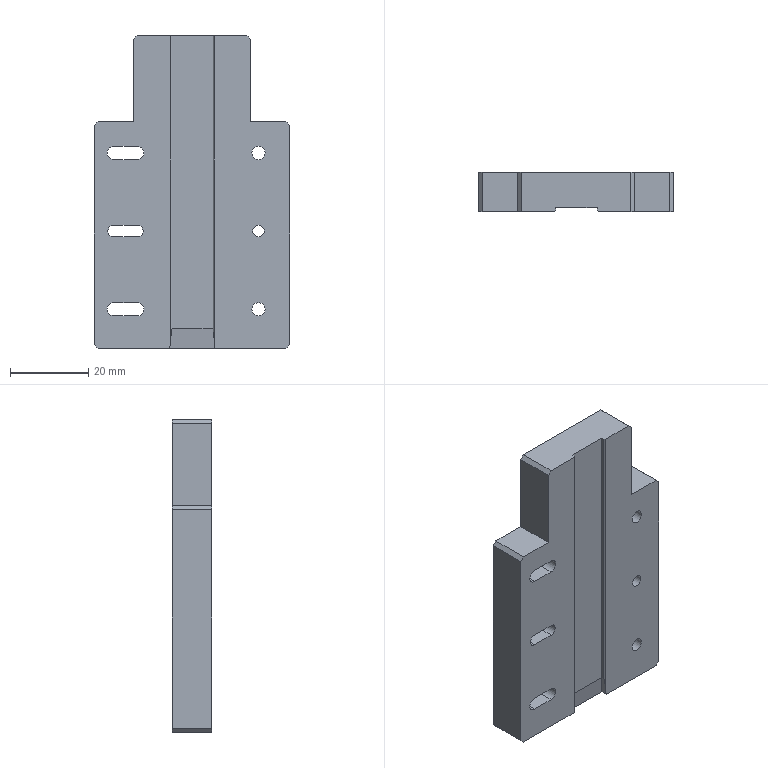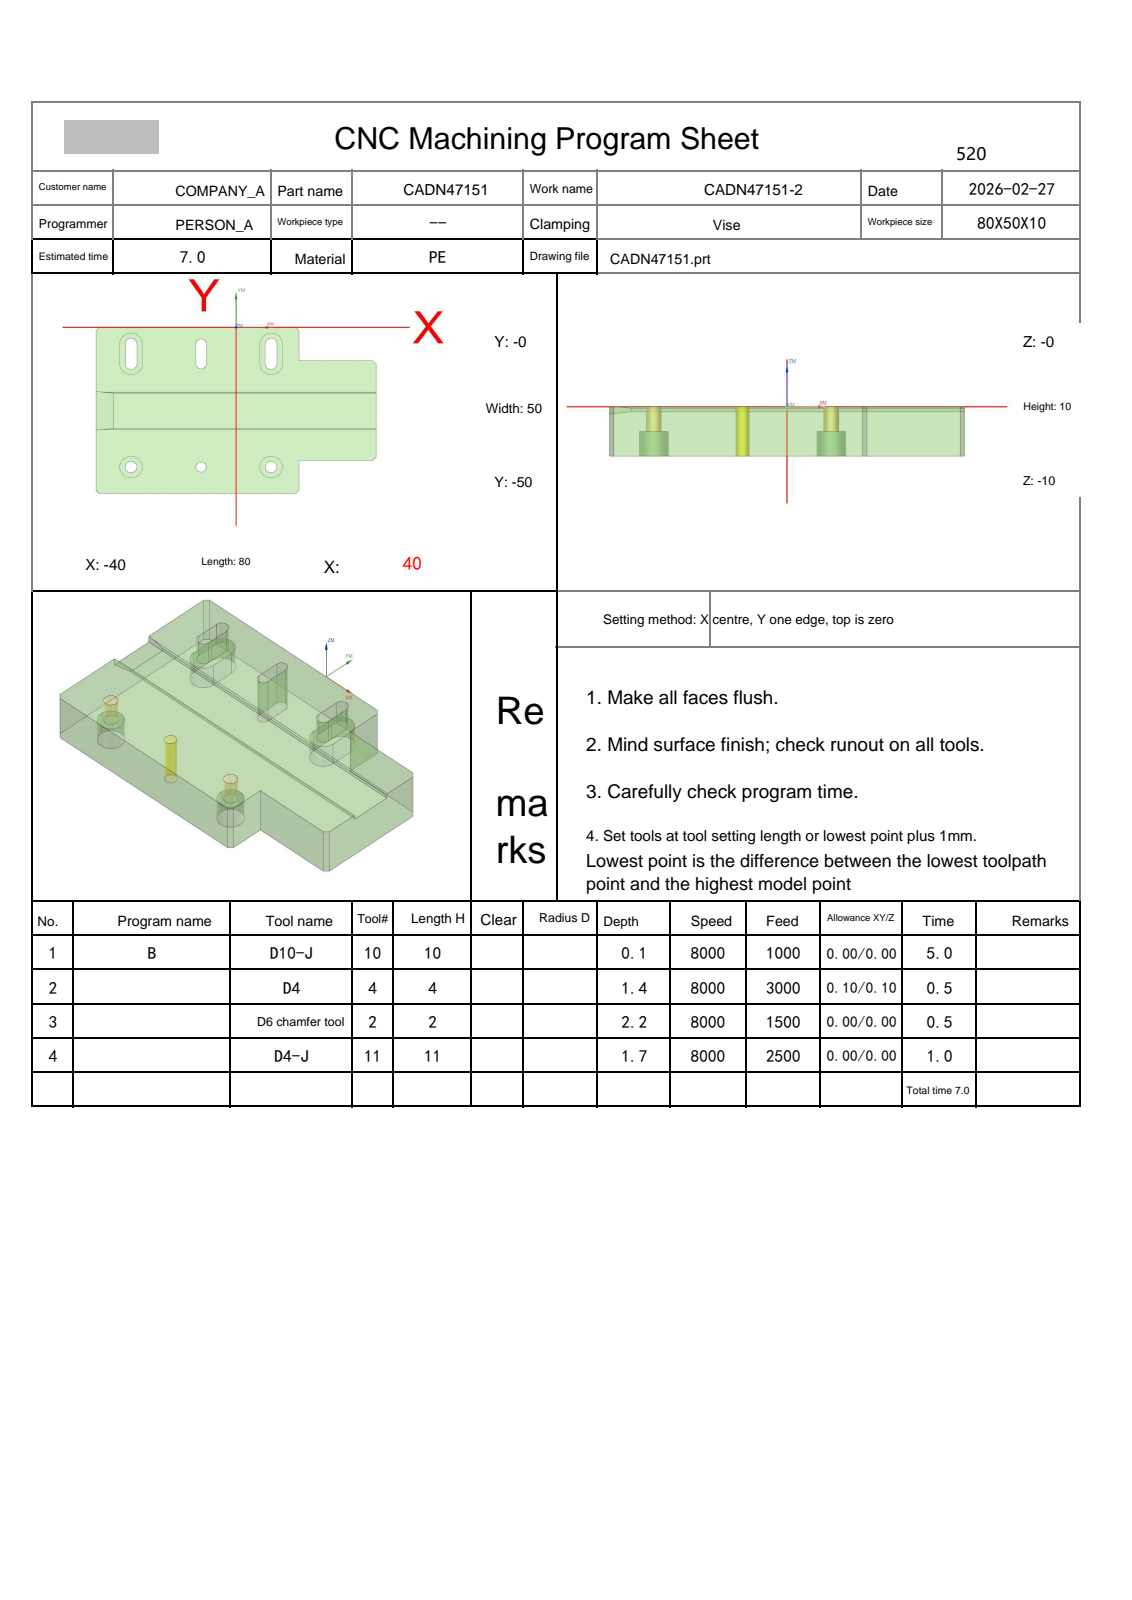NC program | NX | posted by the shop | part box 50 x 10 x 80 mm
Whole program:
%
O0001
(Machine time: 7.76 MIN)
(===Total Tool:4===)
(T10=D10-J  D=10.  R=0.   D-  H10 Z=-0.   )
(T4=D4      D=4.   R=0.   D-  H04 Z=-1.4  )
(T2=D6 chamfer tool   D=6.   R=0.   D-  H02 Z=-2.2  )
(T11=D4-J   D=4.   R=0.   D11 H11 Z=-1.72 )
G80 G90 G17 G49 G40
G91 G28 Z0
M01
N1 T10 M06
(D10-J  D=10. R=0. H=10 ce=0.00 di=0.10)
G00 G90 G54 X-57. Y-16.375 M03 S8000
G43 H10 Z50.
M08
Z3.525
G01 Z1.525 F1000.
X-45. Y-4.375
X-35.625 Y5.
X-26.25
X-45. Y-13.75
Y-23.125
X-16.875 Y5.
X-7.5
X-45. Y-32.5
Y-41.875
X1.875 Y5.
X11.25
X-45. Y-51.25
Y-55.
X-39.375
X20.625 Y5.
X30.
X-30. Y-55.
X-20.625
X39.375 Y5.
X45.
Y1.25
X-11.25 Y-55.
X-1.875
X45. Y-8.125
Y-17.5
X7.5 Y-55.
X16.875
X45. Y-26.875
Y-36.25
X26.25 Y-55.
X35.625
X45. Y-45.625
X57. Y-33.625
Z3.525
G00 Z5.
X-57. Y-16.375
Z3.05
G01 Z1.05
X-45. Y-4.375
X-35.625 Y5.
X-26.25
X-45. Y-13.75
Y-23.125
X-16.875 Y5.
X-7.5
X-45. Y-32.5
Y-41.875
X1.875 Y5.
X11.25
X-45. Y-51.25
Y-55.
X-39.375
X20.625 Y5.
X30.
X-30. Y-55.
X-20.625
X39.375 Y5.
X45.
Y1.25
X-11.25 Y-55.
X-1.875
X45. Y-8.125
Y-17.5
X7.5 Y-55.
X16.875
X45. Y-26.875
Y-36.25
X26.25 Y-55.
X35.625
X45. Y-45.625
X57. Y-33.625
Z3.05
G00 Z4.525
X-57. Y-16.375
Z2.575
G01 Z.575
X-45. Y-4.375
X-35.625 Y5.
X-26.25
X-45. Y-13.75
Y-23.125
X-16.875 Y5.
X-7.5
X-45. Y-32.5
Y-41.875
X1.875 Y5.
X11.25
X-45. Y-51.25
Y-55.
X-39.375
X20.625 Y5.
X30.
X-30. Y-55.
X-20.625
X39.375 Y5.
X45.
Y1.25
X-11.25 Y-55.
X-1.875
X45. Y-8.125
Y-17.5
X7.5 Y-55.
X16.875
X45. Y-26.875
Y-36.25
X26.25 Y-55.
X35.625
X45. Y-45.625
X57. Y-33.625
Z2.575
G00 Z4.05
X-57. Y-16.375
Z2.1
G01 Z.1
X-45. Y-4.375
X-35.625 Y5.
X-26.25
X-45. Y-13.75
Y-23.125
X-16.875 Y5.
X-7.5
X-45. Y-32.5
Y-41.875
X1.875 Y5.
X11.25
X-45. Y-51.25
Y-55.
X-39.375
X20.625 Y5.
X30.
X-30. Y-55.
X-20.625
X39.375 Y5.
X45.
Y1.25
X-11.25 Y-55.
X-1.875
X45. Y-8.125
Y-17.5
X7.5 Y-55.
X16.875
X45. Y-26.875
Y-36.25
X26.25 Y-55.
X35.625
X45. Y-45.625
X57. Y-33.625
Z2.1
G00 Z50.
G00 G90 X-57. Y-16.375 M03 S8000
Z50.
Z2.
G01 Z0.0 F1000.
X-45. Y-4.375
X-35.625 Y5.
X-26.25
X-45. Y-13.75
Y-23.125
X-16.875 Y5.
X-7.5
X-45. Y-32.5
Y-41.875
X1.875 Y5.
X11.25
X-45. Y-51.25
Y-55.
X-39.375
X20.625 Y5.
X30.
X-30. Y-55.
X-20.625
X39.375 Y5.
X45.
Y1.25
X-11.25 Y-55.
X-1.875
X45. Y-8.125
Y-17.5
X7.5 Y-55.
X16.875
X45. Y-26.875
Y-36.25
X26.25 Y-55.
X35.625
X45. Y-45.625
X57. Y-33.625
Z2.
G00 Z50.
G91 G28 Z0.0
M05
M09
G91 G28 Z0.0
M01
N2 T04 M06
(D4  D=4. R=0. H=04 ce=0.10 di=0.10)
G00 G90 G54 X-44.889 Y-27.898 M03 S8000
G43 H04 Z11.8
M08
Z1.
G01 Z-.2 F3000.
X-44.888
G03 X-42.088 Y-25.099 I0.0 J2.8
G01 X-42.086 Y-19.925
X-42.101 Y-19.852
X-42.027 Y-19.848
G03 X-40.209 Y-21.39 I2.027 J.548
G01 X-39.986 Y-21.412
X-39.995 Y-21.49
X-39.913 Y-21.499
X-38.72 Y-21.617
X-38.57 Y-21.632
X-38.138 Y-21.672
X-37.956 Y-21.651
X-37.598
X-35.691 Y-21.841
X39.92
X40.
X40.08
Y-22.017
Y-28.183
Y-28.359
X40.
X39.92
X-35.691
X-37.513 Y-28.541
X-37.998
X-38.186 Y-28.529
X-38.72 Y-28.583
X-39.914 Y-28.701
X-39.995 Y-28.71
X-39.986 Y-28.788
X-40.209 Y-28.81
G03 X-42.024 Y-30.341 I.209 J-2.09
G01 X-42.082 Y-30.339
X-42.059 Y-30.286
X-42.09 Y-30.058
X-42.089 Y-26.617
G02 X-41.884 Y-26.269 I.4 J0.0
G01 X-39.449 Y-24.906
G03 X-39.266 Y-24.687 I-.195 J.349
G02 X-38.888 Y-24.417 I.378 J-.13
G01 X-38.849 Y-24.419
X-38.465 Y-24.457
G03 X-38.259 Y-24.47 I.287 J2.866
G01 X-38.148 Y-24.472
G03 X-37.819 Y-24.453 I0.0 J2.88
G01 X-35.83 Y-24.641
X36.881
G02 X37.28 Y-25.041 I-.001 J-.4
G01 Y-25.159
G02 X36.881 Y-25.559 I-.4 J.001
G01 X-35.83
X-37.672 Y-25.741
X-37.875
G03 X-38.147 Y-25.728 I-.271 J-2.867
G01 X-38.22 Y-25.729
G03 X-38.465 Y-25.743 I.044 J-2.88
G01 X-38.849 Y-25.781
X-38.888 Y-25.783
G02 X-39.288 Y-25.384 I0.0 J.4
G01 Y-24.884
Y-24.883
G03 X-42.087 Y-22.083 I-2.8 J0.0
G01 X-44.887 Y-22.082
Z1.
G00 Z3.
G01 X-44.889 Y-27.898 F6000.
G00 Z.8
G01 Z-.4 F3000.
X-44.888
G03 X-42.088 Y-25.099 I0.0 J2.8
G01 X-42.086 Y-19.925
X-42.101 Y-19.852
X-42.027 Y-19.848
G03 X-40.209 Y-21.39 I2.027 J.548
G01 X-40.068 Y-21.404
X-40.077 Y-21.48
X-39.913 Y-21.499
X-38.72 Y-21.617
X-38.571 Y-21.632
X-38.137 Y-21.671
X-37.956 Y-21.651
X-37.598
X-35.209 Y-21.89
G03 X-35. Y-21.9 I.209 J2.09
G01 X39.92
X40.
X40.008
X40.08
Y-22.017
Y-28.183
Y-28.3
X40.004
X40.
X39.92
X-35.
G03 X-35.209 Y-28.31 I0.0 J-2.1
G01 X-37.513 Y-28.541
X-37.998
X-38.186 Y-28.529
X-38.72 Y-28.583
X-39.914 Y-28.701
X-40.077 Y-28.72
X-40.068 Y-28.796
X-40.209 Y-28.81
G03 X-42.024 Y-30.341 I.209 J-2.09
G01 X-42.082 Y-30.339
X-42.059 Y-30.286
X-42.09 Y-30.058
X-42.089 Y-26.617
G02 X-41.884 Y-26.269 I.4 J0.0
G01 X-39.449 Y-24.906
G03 X-39.266 Y-24.687 I-.196 J.349
G02 X-38.888 Y-24.417 I.378 J-.13
G01 X-38.849 Y-24.419
X-38.465 Y-24.457
G03 X-38.259 Y-24.47 I.287 J2.866
G01 X-38.118 Y-24.474
G03 X-37.756 Y-24.451 I0.0 J2.885
G01 X-35.488 Y-24.676
G03 X-35. Y-24.7 I.488 J4.876
G01 X36.881
G02 X37.28 Y-25.1 I-.001 J-.4
X36.881 Y-25.5 I-.4 J0.0
G01 X-35.
G03 X-35.488 Y-25.524 I0.0 J-4.9
G01 X-37.895 Y-25.739
G03 X-38.147 Y-25.728 I-.252 J-2.869
G01 X-38.22 Y-25.729
G03 X-38.465 Y-25.743 I.044 J-2.88
G01 X-38.849 Y-25.781
X-38.888 Y-25.783
G02 X-39.288 Y-25.384 I0.0 J.4
G01 Y-24.884
Y-24.883
G03 X-42.087 Y-22.083 I-2.8 J0.0
G01 X-44.887 Y-22.082
Z.8
G00 Z2.8
G01 X-44.889 Y-27.898 F6000.
G00 Z.6
G01 Z-.6 F3000.
X-44.888
G03 X-42.088 Y-25.099 I0.0 J2.8
G01 X-42.086 Y-19.925
X-42.101 Y-19.852
X-42.027 Y-19.848
G03 X-40.149 Y-21.396 I2.028 J.548
G01 X-40.158 Y-21.47
X-39.913 Y-21.499
X-38.72 Y-21.617
X-38.571 Y-21.632
X-38.138 Y-21.672
X-37.956 Y-21.651
X-37.598
X-35.209 Y-21.89
G03 X-35. Y-21.9 I.209 J2.09
G01 X39.92
X40.
X40.008
X40.08
Y-22.017
Y-28.183
Y-28.3
X40.004
X40.
X39.92
X-35.
G03 X-35.209 Y-28.31 I0.0 J-2.1
G01 X-37.513 Y-28.541
X-37.998
X-38.186 Y-28.529
X-38.72 Y-28.583
X-39.914 Y-28.701
X-40.158 Y-28.73
X-40.149 Y-28.804
X-40.209 Y-28.81
G03 X-42.024 Y-30.341 I.209 J-2.09
G01 X-42.082 Y-30.339
X-42.059 Y-30.286
X-42.09 Y-30.058
X-42.089 Y-26.617
G02 X-41.884 Y-26.269 I.4 J0.0
G01 X-39.449 Y-24.905
G03 X-39.266 Y-24.687 I-.196 J.349
G02 X-38.888 Y-24.417 I.378 J-.13
G01 X-38.849 Y-24.419
X-38.465 Y-24.457
G03 X-38.259 Y-24.47 I.287 J2.866
G01 X-38.148 Y-24.472
G03 X-37.819 Y-24.453 I0.0 J2.88
G01 X-35.488 Y-24.676
G03 X-35. Y-24.7 I.488 J4.876
G01 X36.881
G02 X37.28 Y-25.1 I-.001 J-.4
X36.881 Y-25.5 I-.4 J0.0
G01 X-35.
G03 X-35.488 Y-25.524 I0.0 J-4.9
G01 X-37.671 Y-25.741
X-37.875
G03 X-38.147 Y-25.728 I-.271 J-2.867
G01 X-38.22 Y-25.729
G03 X-38.465 Y-25.743 I.044 J-2.88
G01 X-38.849 Y-25.782
X-38.888 Y-25.783
G02 X-39.288 Y-25.384 I0.0 J.4
G01 Y-24.884
Y-24.883
G03 X-42.087 Y-22.083 I-2.8 J0.0
G01 X-44.887 Y-22.082
Z.6
G00 Z2.6
G01 X-44.889 Y-27.898 F6000.
G00 Z.4
G01 Z-.8 F3000.
X-44.888
G03 X-42.088 Y-25.099 I0.0 J2.8
G01 X-42.086 Y-19.925
X-42.101 Y-19.852
X-42.027 Y-19.848
G03 X-40.23 Y-21.387 I2.027 J.548
G01 X-40.239 Y-21.461
X-39.913 Y-21.499
X-38.72 Y-21.617
X-38.57 Y-21.632
X-38.138 Y-21.672
X-37.956 Y-21.651
X-37.598
X-35.209 Y-21.89
G03 X-35. Y-21.9 I.209 J2.09
G01 X39.92
X40.
X40.008
X40.08
Y-22.017
Y-28.183
Y-28.3
X40.004
X40.
X39.92
X-35.
G03 X-35.209 Y-28.31 I0.0 J-2.1
G01 X-37.513 Y-28.541
X-37.998
X-38.186 Y-28.529
X-38.72 Y-28.583
X-39.914 Y-28.701
X-40.239 Y-28.739
X-40.23 Y-28.813
G03 X-42.024 Y-30.341 I.23 J-2.087
G01 X-42.082 Y-30.339
X-42.059 Y-30.286
X-42.09 Y-30.058
X-42.089 Y-26.617
G02 X-41.884 Y-26.268 I.4 J0.0
G01 X-39.449 Y-24.906
G03 X-39.266 Y-24.687 I-.195 J.349
G02 X-38.888 Y-24.417 I.378 J-.13
G01 X-38.849 Y-24.419
X-38.465 Y-24.457
G03 X-38.259 Y-24.47 I.287 J2.866
G01 X-38.148 Y-24.472
G03 X-37.819 Y-24.453 I0.0 J2.88
G01 X-35.488 Y-24.676
G03 X-35. Y-24.7 I.488 J4.876
G01 X36.881
G02 X37.28 Y-25.1 I-.001 J-.4
X36.881 Y-25.5 I-.4 J0.0
G01 X-35.
G03 X-35.488 Y-25.524 I0.0 J-4.9
G01 X-37.672 Y-25.741
X-37.875
G03 X-38.147 Y-25.728 I-.271 J-2.867
G01 X-38.22 Y-25.729
G03 X-38.465 Y-25.743 I.044 J-2.88
G01 X-38.849 Y-25.781
X-38.888 Y-25.783
G02 X-39.288 Y-25.384 I0.0 J.4
G01 Y-24.884
Y-24.883
G03 X-42.087 Y-22.083 I-2.8 J0.0
G01 X-44.887 Y-22.082
Z.4
G00 Z2.4
G01 X-44.889 Y-27.898 F6000.
G00 Z.2
G01 Z-1. F3000.
X-44.888
G03 X-42.088 Y-25.099 I0.0 J2.8
G01 X-42.086 Y-19.925
X-42.101 Y-19.852
X-42.027 Y-19.848
G03 X-40.311 Y-21.377 I2.027 J.548
G01 X-40.32 Y-21.451
X-39.805 Y-21.51
X-38.72 Y-21.617
X-38.138 Y-21.672
X-38.005 Y-21.656
Y-28.54
X-38.186 Y-28.529
X-38.72 Y-28.583
X-39.914 Y-28.701
X-40.32 Y-28.749
X-40.311 Y-28.823
G03 X-42.024 Y-30.341 I.311 J-2.077
G01 X-42.082 Y-30.339
X-42.059 Y-30.286
X-42.09 Y-30.058
X-42.088 Y-26.164
G02 X-41.971 Y-25.882 I.4 J0.0
G01 X-40.405 Y-24.316
G03 X-40.288 Y-24.034 I-.283 J.283
G01 X-40.287 Y-23.535
G02 X-40.047 Y-23.296 I.24 J-.001
G01 X-40.021 Y-23.298
G02 X-39.805 Y-23.536 I-.024 J-.239
G01 Y-26.664
G02 X-40.026 Y-26.903 I-.24 J.001
G01 X-40.049 Y-26.904
G02 X-40.289 Y-26.665 I0.0 J.24
G01 X-40.288 Y-25.099
Y-24.599
Y-24.598
G03 X-43.087 Y-21.798 I-2.8 J0.0
G01 X-44.887
Z.2
G00 Z2.2
G01 X-44.889 Y-27.898 F6000.
G00 Z0.0
G01 Z-1.2 F3000.
X-44.888
G03 X-42.088 Y-25.099 I0.0 J2.8
G01 X-42.086 Y-19.925
X-42.101 Y-19.852
X-42.027 Y-19.848
G03 X-40.392 Y-21.363 I2.027 J.548
G01 X-40.401 Y-21.441
X-40.005 Y-21.488
Y-28.712
X-40.401 Y-28.759
X-40.392 Y-28.837
G03 X-42.024 Y-30.341 I.392 J-2.063
G01 X-42.082 Y-30.339
X-42.059 Y-30.286
X-42.09 Y-30.058
X-42.088 Y-25.099
Y-24.599
Y-24.598
G03 X-44.887 Y-21.798 I-2.8 J0.0
G01 Z0.0
G00 Z2.
G01 X-44.889 Y-27.898 F6000.
G00 Z-.2
G01 Z-1.4 F3000.
X-44.888
G03 X-42.088 Y-25.099 I0.0 J2.8
G01 X-42.086 Y-20.647
X-42.005 Y-20.648
Y-29.552
X-42.09
X-42.088 Y-25.099
Y-24.599
Y-24.598
G03 X-44.887 Y-21.798 I-2.8 J0.0
G01 Z-.2
G00 Z11.8
G91 G28 Z0.0
M05
M09
G91 G28 Z0.0
M01
N3 T02 M06
(D6 chamfer tool  D=6. R=0. H=02 ce=0.00 di=0.10)
G00 G90 G54 X-10. Y-42. M03 S8000
G43 H02 Z50.
M08
G98 G81 X-10. Y-42. Z-1.8 R3. F1000.
G80
G00 Z50.
G00 G90 X-30. Y-42. M03 S8000
Z50.
G98 G81 X-30. Y-42. Z-2. R3. F1000.
X10.
G80
G00 Z50.
G00 G90 X-37.333 Y-20.5 M03 S6500
Z50.
Z2.8
G01 Z-1.2 F1500.
X-38.
X-38.05 Y-20.499
X-40.1 Y-20.295
G02 X-41. Y-19.3 I.1 J.995
G01 Y-1.
X-40.966 Y-.741
X-40.866 Y-.5
X-40.707 Y-.293
X-39.707 Y.707
X-39.5 Y.866
X-39.259 Y.966
X-39. Y1.
X17.
X17.259 Y.966
X17.5 Y.866
X17.707 Y.707
X18.707 Y-.293
X18.866 Y-.5
X18.966 Y-.741
X19. Y-1.
Y-9.
X39.
X39.259 Y-9.034
X39.5 Y-9.134
X39.707 Y-9.293
X40.707 Y-10.293
X40.866 Y-10.5
X40.966 Y-10.741
X41. Y-11.
Y-19.5
X40.966 Y-19.759
X40.928 Y-19.849
X40.905 Y-19.898
X40.915 Y-19.952
G03 X40.99 Y-20.292 I1.983 J.261
G01 Z.13
G00 Z10.
X-30.473 Y-7.614
Z.172
G01 Z-1.2
G03 X-30.673 Y-7.9 I1.532 J-1.286
G01 X-30.703 Y-7.946
X-30.7 Y-8.
Y-11.
G03 X-30. Y-11.7 I.7 J0.0
X-29.784 Y-11.666 I0.0 J.7
G01 X-29.589 Y-11.566
X-29.434 Y-11.411
X-29.334 Y-11.216
X-29.3 Y-11.
Y-5.
G03 X-30. Y-4.3 I-.7 J0.0
X-30.216 Y-4.334 I0.0 J-.7
G01 X-30.411 Y-4.434
X-30.566 Y-4.589
X-30.666 Y-4.784
X-30.7 Y-5.
Y-8.
X-30.703 Y-8.054
X-30.673 Y-8.1
G03 X-30.473 Y-8.386 I1.732 J1.
G01 Z.172
G00 Z10.
X-10.273 Y-7.614
Z.172
G01 Z-1.2
G03 X-10.473 Y-7.9 I1.532 J-1.286
G01 X-10.503 Y-7.946
X-10.5 Y-8.
Y-11.
G03 X-10. Y-11.5 I.5 J0.0
G01 X-9.809 Y-11.462
X-9.646 Y-11.354
X-9.538 Y-11.191
X-9.5 Y-11.
Y-5.
G03 X-10. Y-4.5 I-.5 J0.0
G01 X-10.191 Y-4.538
X-10.354 Y-4.646
X-10.462 Y-4.809
X-10.5 Y-5.
Y-8.
X-10.503 Y-8.054
X-10.473 Y-8.1
G03 X-10.273 Y-8.386 I1.732 J1.
G01 Z.172
G00 Z10.
X9.527 Y-7.614
Z.172
G01 Z-1.2
G03 X9.327 Y-7.9 I1.532 J-1.286
G01 X9.297 Y-7.946
X9.3 Y-8.
Y-11.
G03 X10. Y-11.7 I.7 J0.0
X10.216 Y-11.666 I0.0 J.7
G01 X10.411 Y-11.566
X10.566 Y-11.411
X10.666 Y-11.216
X10.7 Y-11.
Y-5.
G03 X10. Y-4.3 I-.7 J0.0
X9.784 Y-4.334 I0.0 J-.7
G01 X9.589 Y-4.434
X9.434 Y-4.589
X9.334 Y-4.784
X9.3 Y-5.
Y-8.
X9.297 Y-8.054
X9.327 Y-8.1
G03 X9.527 Y-8.386 I1.732 J1.
G01 Z.172
G00 Z10.
X40.99 Y-29.908
Z.13
G01 Z-1.2
G03 X40.915 Y-30.248 I1.907 J-.601
G01 X40.905 Y-30.302
X40.928 Y-30.351
X40.966 Y-30.441
X41. Y-30.7
Y-39.
X40.966 Y-39.259
X40.866 Y-39.5
X40.707 Y-39.707
X39.707 Y-40.707
X39.5 Y-40.866
X39.259 Y-40.966
X39. Y-41.
X19.
Y-49.
X18.966 Y-49.259
X18.866 Y-49.5
X18.707 Y-49.707
X17.707 Y-50.707
X17.5 Y-50.866
X17.259 Y-50.966
X17. Y-51.
X-39.
X-39.259 Y-50.966
X-39.5 Y-50.866
X-39.707 Y-50.707
X-40.707 Y-49.707
X-40.866 Y-49.5
X-40.966 Y-49.259
X-41. Y-49.
Y-30.9
G02 X-40.1 Y-29.905 I1. J0.0
G01 X-38.05 Y-29.701
X-37.306 Y-29.7
Z2.8
G00 Z10.
X-29.474 Y-42.412
Z.375
G01 Z-1.2
G03 X-29.314 Y-42.103 I-1.687 J1.075
G01 X-29.29 Y-42.054
X-29.3 Y-42.
G03 X-30. Y-41.3 I-.7 J0.0
X-30.7 Y-42. I0.0 J-.7
X-30. Y-42.7 I.7 J0.0
X-29.324 Y-42.181 I0.0 J.7
G01 X-29.3 Y-42.
X-29.29 Y-41.946
X-29.314 Y-41.897
G03 X-29.474 Y-41.588 I-1.848 J-.765
G01 Z.376
G00 Z10.
X-9.656 Y-42.419
Z.447
G01 Z-1.2
G03 X-9.509 Y-42.103 I-1.732 J1.
G01 X-9.488 Y-42.053
X-9.5 Y-42.
G03 X-10. Y-41.5 I-.5 J0.0
X-10.5 Y-42. I0.0 J-.5
X-10. Y-42.5 I.5 J0.0
X-9.5 Y-42. I0.0 J.5
G01 X-9.488 Y-41.947
X-9.509 Y-41.897
G03 X-9.656 Y-41.581 I-1.879 J-.684
G01 Z.447
G00 Z10.
X10.526 Y-42.412
Z.375
G01 Z-1.2
G03 X10.686 Y-42.103 I-1.687 J1.075
G01 X10.71 Y-42.054
X10.7 Y-42.
G03 X10. Y-41.3 I-.7 J0.0
X9.3 Y-42. I0.0 J-.7
X10. Y-42.7 I.7 J0.0
X10.676 Y-42.181 I0.0 J.7
G01 X10.7 Y-42.
X10.71 Y-41.946
X10.686 Y-41.897
G03 X10.526 Y-41.588 I-1.848 J-.765
G01 Z.376
G00 Z10.
X41. Y-21.456
Z1.8
G01 Z-2.2
Y-28.77
Z1.8
G00 Z50.
G00 G90 X43.963 Y-21.4 M03 S6500
Z50.
Z.8
G01 Z-.7 F1500.
G03 X42.763 Y-20.2 I-1.2 J0.0
G01 X-40.867
G03 X-41.9 Y-20.79 I0.0 J-1.2
G01 Z.8
G00 Y-29.375
G01 Z-.7
G03 X-40.847 Y-30. I1.053 J.575
G01 X42.763
G03 X43.963 Y-28.8 I0.0 J1.2
G01 Z.8
G00 Z50.
G91 G28 Z0.0
M05
M09
G91 G28 Z0.0
M01
N4 T11 M06
(D4-J  D=4. R=0. H=11 ce=0.40 di=0.00)
G00 G90 G54 X42.8 Y-24.3 M03 S8000
G43 H11 Z11.8
M08
Z.5
G01 Z-1. F800.
X41.2
G03 X40.4 Y-25.1 I0.0 J-.8
G01 Y-27.602
G02 X40.002 Y-28. I-.4 J.002
G01 X-35.081
G02 X-35.4 Y-27.681 I.001 J.32
G01 Y-22.519
G02 X-35.081 Y-22.2 I.32 J-.001
G01 X40.002
G02 X40.4 Y-22.598 I-.002 J-.4
G01 Y-27.1
G02 X40. Y-27.5 I-.4 J0.0
X39.793 Y-27.442 I0.0 J.4
G01 X37.5 Y-26.057
G03 X37.294 Y-26. I-.206 J-.343
G01 X-33.002
G02 X-33.4 Y-25.602 I.002 J.4
G01 Y-24.598
G02 X-33.002 Y-24.2 I.4 J-.002
G01 X38.002
G02 X38.4 Y-24.598 I-.002 J-.4
G01 Y-25.602
G02 X38.339 Y-25.812 I-.4 J.002
X38.002 Y-26. I-.339 J.212
G01 X37.405
G03 X36.605 Y-26.8 I0.0 J-.8
G01 Z.5
G00 Z11.8
G00 G90 X42.8 Y-22.8 M03 S8000
Z11.8
Z0.0
G01 Z-1. F800.
G41 D11
Y-22.6
G03 X42. Y-21.8 I-.8 J0.0
G01 X-35.1
X-37. Y-21.61
X-37.08 Y-21.606
G03 X-37.876 Y-22.326 I0.0 J-.8
G01 G40 X-37.896 Y-22.525
Z0.0
G00 Y-27.675
G01 Z-1.
G41 D11
X-37.876 Y-27.874
G03 X-37.08 Y-28.594 I.796 J.08
G01 X-37. Y-28.59
X-35.1 Y-28.4
X42.
G03 X42.8 Y-27.6 I0.0 J.8
G01 G40 Y-27.4
Z0.0
G00 Z11.8
G00 G90 X-33.03 Y-22.007 M03 S5000
Z50.
Z2.
G01 Z-.7 F2500.
X-36.999 Y-21.61 Z-1.
X-40.197 Y-21.29 Z-1.32
X-44.158 Y-20.894 Z-1.716
Z1.2
G00 Z50.
Y-29.306
Z1.2
G01 Z-1.716
X-40.197 Y-28.91 Z-1.32
X-37.004 Y-28.59 Z-1.
X-36.999
X-33.03 Y-28.193 Z-.7
Z2.
G00 Z50.
G00 G90 X-39.317 Y-26.802 M03 S7000
Z11.8
Z-.504
G01 Z-1.004 F2500.
X-39.313 Y-26.84
G03 X-37.327 Y-28.603 I1.986 J.237
X-37.09 Y-28.589 I0.0 J2.
G01 X-36.96 Y-28.573
Y-21.627
X-37.09 Y-21.611
Z-1.008
Y-28.589
X-37.13 Y-28.593 Z-1.012
Y-21.607
X-37.17 Y-21.603 Z-1.016
Y-28.597
X-37.21 Y-28.601 Z-1.02
Y-21.599
X-37.25 Y-21.595 Z-1.024
Y-28.605
X-37.29 Y-28.609 Z-1.028
Y-21.591
X-37.33 Y-21.587 Z-1.032
Y-28.613
X-37.37 Y-28.617 Z-1.036
Y-21.583
X-37.41 Y-21.579 Z-1.04
Y-28.621
X-37.45 Y-28.625 Z-1.044
Y-21.575
X-37.49 Y-21.571 Z-1.048
Y-28.629
X-37.53 Y-28.633 Z-1.052
Y-21.567
X-37.57 Y-21.563 Z-1.056
Y-28.637
X-37.61 Y-28.641 Z-1.06
Y-21.559
X-37.65 Y-21.555 Z-1.064
Y-28.645
X-37.69 Y-28.649 Z-1.068
Y-21.551
X-37.73 Y-21.547 Z-1.072
Y-28.653
X-37.77 Y-28.657 Z-1.076
Y-21.543
X-37.81 Y-21.539 Z-1.08
Y-28.661
X-37.85 Y-28.665 Z-1.084
Y-21.535
X-37.89 Y-21.531 Z-1.088
Y-28.669
X-37.93 Y-28.673 Z-1.092
Y-21.527
X-37.97 Y-21.523 Z-1.096
Y-28.677
X-38.01 Y-28.681 Z-1.1
Y-21.519
X-38.05 Y-21.515 Z-1.104
Y-28.685
X-38.09 Y-28.689 Z-1.108
Y-21.511
X-38.13 Y-21.507 Z-1.112
Y-28.693
X-38.17 Y-28.697 Z-1.116
Y-21.503
X-38.21 Y-21.499 Z-1.12
Y-28.701
X-38.25 Y-28.705 Z-1.124
Y-21.495
X-38.29 Y-21.491 Z-1.128
Y-28.709
X-38.33 Y-28.713 Z-1.132
Y-21.487
X-38.37 Y-21.483 Z-1.136
Y-28.717
X-38.41 Y-28.721 Z-1.14
Y-21.479
X-38.45 Y-21.475 Z-1.144
Y-28.725
X-38.49 Y-28.729 Z-1.148
Y-21.471
X-38.53 Y-21.467 Z-1.152
Y-28.733
X-38.57 Y-28.737 Z-1.156
Y-21.463
X-38.61 Y-21.459 Z-1.16
Y-28.741
X-38.65 Y-28.745 Z-1.164
Y-21.455
X-38.69 Y-21.451 Z-1.168
Y-28.749
X-38.73 Y-28.753 Z-1.172
Y-21.447
X-38.77 Y-21.443 Z-1.176
Y-28.757
X-38.81 Y-28.761 Z-1.18
Y-21.439
X-38.85 Y-21.435 Z-1.184
Y-28.765
X-38.89 Y-28.769 Z-1.188
Y-21.431
X-38.93 Y-21.427 Z-1.192
Y-28.773
X-38.97 Y-28.777 Z-1.196
Y-21.423
X-39.01 Y-21.419 Z-1.2
Y-28.781
X-39.05 Y-28.785 Z-1.204
Y-21.415
X-39.09 Y-21.411 Z-1.208
Y-28.789
X-39.13 Y-28.793 Z-1.212
Y-21.407
X-39.17 Y-21.403 Z-1.216
Y-28.797
X-39.21 Y-28.801 Z-1.22
Y-21.399
X-39.25 Y-21.395 Z-1.224
Y-28.805
X-39.29 Y-28.809 Z-1.228
Y-21.391
X-39.33 Y-21.387 Z-1.232
Y-28.813
X-39.37 Y-28.817 Z-1.236
Y-21.383
X-39.41 Y-21.379 Z-1.24
Y-28.821
X-39.45 Y-28.825 Z-1.244
Y-21.375
X-39.49 Y-21.371 Z-1.248
Y-28.829
X-39.53 Y-28.833 Z-1.252
Y-21.367
X-39.57 Y-21.363 Z-1.256
Y-28.837
X-39.61 Y-28.841 Z-1.26
Y-21.359
X-39.65 Y-21.355 Z-1.264
Y-28.845
X-39.69 Y-28.849 Z-1.268
Y-21.351
X-39.73 Y-21.347 Z-1.272
Y-28.853
X-39.77 Y-28.857 Z-1.276
Y-21.343
X-39.81 Y-21.339 Z-1.28
Y-28.861
X-39.85 Y-28.865 Z-1.284
Y-21.335
X-39.89 Y-21.331 Z-1.288
Y-28.869
X-39.93 Y-28.873 Z-1.292
Y-21.327
X-39.97 Y-21.323 Z-1.296
Y-28.877
X-40.01 Y-28.89 Z-1.3
Y-21.319
X-40.05 Y-21.315 Z-1.304
Y-28.891
X-40.09 Y-28.892 Z-1.308
Y-21.308
X-40.13 Y-21.306 Z-1.312
Y-28.894
X-40.17 Y-28.897 Z-1.316
Y-21.303
X-40.21 Y-21.299 Z-1.32
Y-28.901
X-40.25 Y-28.906 Z-1.324
Y-21.294
X-40.29 Y-21.289 Z-1.328
Y-28.911
X-40.33 Y-28.917 Z-1.332
Y-21.283
X-40.37 Y-21.276 Z-1.336
Y-28.924
X-40.41 Y-28.932 Z-1.34
Y-21.268
X-40.45 Y-21.259 Z-1.344
Y-28.941
X-40.49 Y-28.951 Z-1.348
Y-21.249
X-40.53 Y-21.239 Z-1.352
Y-28.961
X-40.57 Y-28.973 Z-1.356
Y-21.227
X-40.61 Y-21.215 Z-1.36
Y-28.985
X-40.65 Y-28.998 Z-1.364
Y-21.202
X-40.69 Y-21.188 Z-1.368
Y-29.012
X-40.73 Y-29.027 Z-1.372
Y-21.173
X-40.77 Y-21.157 Z-1.376
Y-29.043
X-40.81 Y-29.06 Z-1.38
Y-21.14
X-40.85 Y-21.121 Z-1.384
Y-29.079
X-40.89 Y-29.098 Z-1.388
Y-21.102
X-40.93 Y-21.082 Z-1.392
Y-29.118
X-40.97 Y-29.14 Z-1.396
Y-21.06
X-41.01 Y-21.038 Z-1.4
Y-29.162
X-41.05 Y-29.186 Z-1.404
Y-21.014
X-41.09 Y-20.989 Z-1.408
Y-29.211
X-41.13 Y-29.238 Z-1.412
Y-20.962
X-41.17 Y-20.934 Z-1.416
Y-29.266
X-41.21 Y-29.295 Z-1.42
Y-20.905
X-41.25 Y-20.874 Z-1.424
Y-29.326
X-41.29 Y-29.359 Z-1.428
Y-20.841
X-41.33 Y-20.807 Z-1.432
Y-29.393
X-41.37 Y-29.429 Z-1.436
Y-20.771
X-41.41 Y-20.732 Z-1.44
Y-29.468
X-41.45 Y-29.508 Z-1.444
Y-20.692
X-41.49 Y-20.649 Z-1.448
Y-29.551
X-41.53 Y-29.596 Z-1.452
Y-20.604
X-41.57 Y-20.555 Z-1.456
Y-29.645
X-41.61 Y-29.697 Z-1.46
Y-20.503
X-41.65 Y-20.448 Z-1.464
Y-29.752
X-41.69 Y-29.812 Z-1.468
Y-20.388
X-41.73 Y-20.323 Z-1.472
Y-29.877
X-41.77 Y-29.948 Z-1.476
Y-20.252
X-41.81 Y-20.174 Z-1.48
Y-30.026
X-41.85 Y-30.114 Z-1.484
Y-20.086
X-41.89 Y-19.984 Z-1.488
Y-30.216
G00 Z-1.
X-44.01 Y-32.9
G01 Z-1.5
G03 X-42.01 Y-30.9 I0.0 J2.
G01 Y-19.3
G00 Z11.8
M05
M09
G91 G28 Z0.0
G91 G28 Y0.0
M30
%